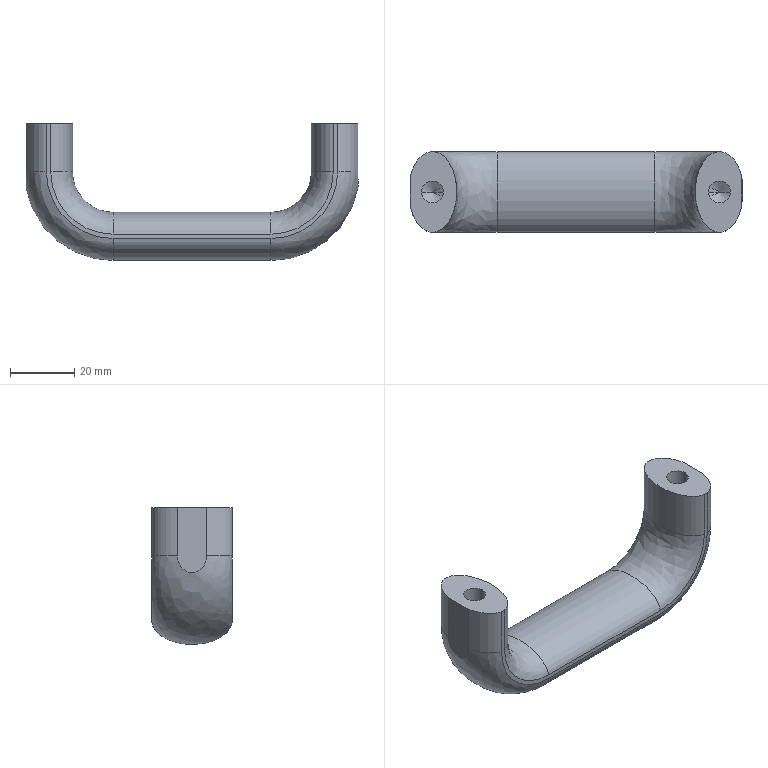Part | SolidWorks | features CutThin 1, HoleWzd 1, Sweep 1 | 1 solid | 26 faces | box 103 x 24.9 x 42.5 mm | volume 40167 mm3 | spline 12 | plane 6 | cylinder 4 | cone 4 | commonest cylinder face diameters 6.8 x4
STEP:
#1=CARTESIAN_POINT('',(-3.4,0.,-19.75));
#2=VERTEX_POINT('',#1);
#3=CARTESIAN_POINT('',(3.4,0.,-19.75));
#4=VERTEX_POINT('',#3);
#5=CARTESIAN_POINT('',(0.,0.,-19.75));
#6=DIRECTION('',(0.,0.,1.));
#7=DIRECTION('',(1.,0.,0.));
#8=AXIS2_PLACEMENT_3D('',#5,#6,#7);
#9=CIRCLE('',#8,3.4);
#10=EDGE_CURVE('',#2,#4,#9,.T.);
#11=ORIENTED_EDGE('',*,*,#10,.F.);
#12=CARTESIAN_POINT('',(-3.4,0.,0.));
#13=VERTEX_POINT('',#12);
#14=CARTESIAN_POINT('',(-3.4,0.,0.));
#15=DIRECTION('',(0.,0.,1.));
#16=VECTOR('',#15,1000.);
#17=LINE('',#14,#16);
#18=EDGE_CURVE('',#2,#13,#17,.T.);
#19=ORIENTED_EDGE('',*,*,#18,.T.);
#20=CARTESIAN_POINT('',(3.4,0.,0.));
#21=VERTEX_POINT('',#20);
#22=CARTESIAN_POINT('',(0.,0.,0.));
#23=DIRECTION('',(0.,0.,1.));
#24=DIRECTION('',(1.,0.,0.));
#25=AXIS2_PLACEMENT_3D('',#22,#23,#24);
#26=CIRCLE('',#25,3.4);
#27=EDGE_CURVE('',#13,#21,#26,.T.);
#28=ORIENTED_EDGE('',*,*,#27,.T.);
#29=CARTESIAN_POINT('',(3.4,0.,0.));
#30=DIRECTION('',(0.,0.,1.));
#31=VECTOR('',#30,1000.);
#32=LINE('',#29,#31);
#33=EDGE_CURVE('',#4,#21,#32,.T.);
#34=ORIENTED_EDGE('',*,*,#33,.F.);
#35=EDGE_LOOP('',(#11,#19,#28,#34));
#36=FACE_OUTER_BOUND('',#35,.T.);
#37=CARTESIAN_POINT('',(0.,0.,0.));
#38=DIRECTION('',(0.,0.,1.));
#39=DIRECTION('',(1.,0.,0.));
#40=AXIS2_PLACEMENT_3D('',#37,#38,#39);
#41=CYLINDRICAL_SURFACE('',#40,3.4);
#42=ADVANCED_FACE('',(#36),#41,.F.);
#43=CARTESIAN_POINT('',(0.,0.,-21.793));
#44=VERTEX_POINT('',#43);
#45=CARTESIAN_POINT('',(3.4,0.,-19.75));
#46=DIRECTION('',(0.8572,0.,0.515));
#47=VECTOR('',#46,1000.);
#48=LINE('',#45,#47);
#49=EDGE_CURVE('',#44,#4,#48,.T.);
#50=ORIENTED_EDGE('',*,*,#49,.F.);
#51=CARTESIAN_POINT('',(-3.4,0.,-19.75));
#52=DIRECTION('',(-0.8572,0.,0.515));
#53=VECTOR('',#52,1000.);
#54=LINE('',#51,#53);
#55=EDGE_CURVE('',#44,#2,#54,.T.);
#56=ORIENTED_EDGE('',*,*,#55,.T.);
#57=ORIENTED_EDGE('',*,*,#10,.T.);
#58=EDGE_LOOP('',(#50,#56,#57));
#59=FACE_OUTER_BOUND('',#58,.T.);
#60=CARTESIAN_POINT('',(0.,0.,-19.75));
#61=DIRECTION('',(0.,0.,1.));
#62=DIRECTION('',(1.,0.,0.));
#63=AXIS2_PLACEMENT_3D('',#60,#61,#62);
#64=CONICAL_SURFACE('',#63,3.4,1.03);
#65=ADVANCED_FACE('',(#59),#64,.F.);
#66=CARTESIAN_POINT('',(85.6,0.,-19.75));
#67=VERTEX_POINT('',#66);
#68=CARTESIAN_POINT('',(92.4,0.,-19.75));
#69=VERTEX_POINT('',#68);
#70=CARTESIAN_POINT('',(89.,0.,-19.75));
#71=DIRECTION('',(0.,0.,1.));
#72=DIRECTION('',(1.,0.,0.));
#73=AXIS2_PLACEMENT_3D('',#70,#71,#72);
#74=CIRCLE('',#73,3.4);
#75=EDGE_CURVE('',#67,#69,#74,.T.);
#76=ORIENTED_EDGE('',*,*,#75,.F.);
#77=CARTESIAN_POINT('',(85.6,0.,0.));
#78=VERTEX_POINT('',#77);
#79=CARTESIAN_POINT('',(85.6,0.,0.));
#80=DIRECTION('',(0.,0.,1.));
#81=VECTOR('',#80,1000.);
#82=LINE('',#79,#81);
#83=EDGE_CURVE('',#67,#78,#82,.T.);
#84=ORIENTED_EDGE('',*,*,#83,.T.);
#85=CARTESIAN_POINT('',(92.4,0.,0.));
#86=VERTEX_POINT('',#85);
#87=CARTESIAN_POINT('',(89.,0.,0.));
#88=DIRECTION('',(0.,0.,1.));
#89=DIRECTION('',(1.,0.,0.));
#90=AXIS2_PLACEMENT_3D('',#87,#88,#89);
#91=CIRCLE('',#90,3.4);
#92=EDGE_CURVE('',#78,#86,#91,.T.);
#93=ORIENTED_EDGE('',*,*,#92,.T.);
#94=CARTESIAN_POINT('',(92.4,0.,0.));
#95=DIRECTION('',(0.,0.,1.));
#96=VECTOR('',#95,1000.);
#97=LINE('',#94,#96);
#98=EDGE_CURVE('',#69,#86,#97,.T.);
#99=ORIENTED_EDGE('',*,*,#98,.F.);
#100=EDGE_LOOP('',(#76,#84,#93,#99));
#101=FACE_OUTER_BOUND('',#100,.T.);
#102=CARTESIAN_POINT('',(89.,0.,0.));
#103=DIRECTION('',(0.,0.,1.));
#104=DIRECTION('',(1.,0.,0.));
#105=AXIS2_PLACEMENT_3D('',#102,#103,#104);
#106=CYLINDRICAL_SURFACE('',#105,3.4);
#107=ADVANCED_FACE('',(#101),#106,.F.);
#108=CARTESIAN_POINT('',(89.,0.,-21.793));
#109=VERTEX_POINT('',#108);
#110=CARTESIAN_POINT('',(92.4,0.,-19.75));
#111=DIRECTION('',(0.8572,0.,0.515));
#112=VECTOR('',#111,1000.);
#113=LINE('',#110,#112);
#114=EDGE_CURVE('',#109,#69,#113,.T.);
#115=ORIENTED_EDGE('',*,*,#114,.F.);
#116=CARTESIAN_POINT('',(85.6,0.,-19.75));
#117=DIRECTION('',(-0.8572,0.,0.515));
#118=VECTOR('',#117,1000.);
#119=LINE('',#116,#118);
#120=EDGE_CURVE('',#109,#67,#119,.T.);
#121=ORIENTED_EDGE('',*,*,#120,.T.);
#122=ORIENTED_EDGE('',*,*,#75,.T.);
#123=EDGE_LOOP('',(#115,#121,#122));
#124=FACE_OUTER_BOUND('',#123,.T.);
#125=CARTESIAN_POINT('',(89.,0.,-19.75));
#126=DIRECTION('',(0.,0.,1.));
#127=DIRECTION('',(1.,0.,0.));
#128=AXIS2_PLACEMENT_3D('',#125,#126,#127);
#129=CONICAL_SURFACE('',#128,3.4,1.03);
#130=ADVANCED_FACE('',(#124),#129,.F.);
#131=CARTESIAN_POINT('',(89.,0.,0.));
#132=DIRECTION('',(0.,0.,1.));
#133=DIRECTION('',(1.,0.,0.));
#134=AXIS2_PLACEMENT_3D('',#131,#132,#133);
#135=CIRCLE('',#134,3.4);
#136=EDGE_CURVE('',#86,#78,#135,.T.);
#137=ORIENTED_EDGE('',*,*,#136,.F.);
#138=ORIENTED_EDGE('',*,*,#92,.F.);
#139=EDGE_LOOP('',(#137,#138));
#140=FACE_BOUND('',#139,.T.);
#141=CARTESIAN_POINT('',(96.,-4.488,0.));
#142=VERTEX_POINT('',#141);
#143=CARTESIAN_POINT('',(96.,4.488,0.));
#144=VERTEX_POINT('',#143);
#145=CARTESIAN_POINT('',(96.,-12.45,0.));
#146=DIRECTION('',(0.,1.,0.));
#147=VECTOR('',#146,1000.);
#148=LINE('',#145,#147);
#149=EDGE_CURVE('',#142,#144,#148,.T.);
#150=ORIENTED_EDGE('',*,*,#149,.T.);
#151=CARTESIAN_POINT('',(89.67,12.45,0.));
#152=VERTEX_POINT('',#151);
#153=CARTESIAN_POINT('',(89.67,12.45,0.));
#154=CARTESIAN_POINT('',(92.598,12.012,0.));
#155=CARTESIAN_POINT('',(94.945,9.061,0.));
#156=CARTESIAN_POINT('',(96.,4.488,0.));
#157=(BOUNDED_CURVE()B_SPLINE_CURVE(3,(#153,#154,#155,#156),.UNSPECIFIED.,.F.,.F.)B_SPLINE_CURVE_WITH_KNOTS((4,4),(0.08947,1.204),.UNSPECIFIED.)CURVE()GEOMETRIC_REPRESENTATION_ITEM()RATIONAL_B_SPLINE_CURVE((1.,0.8992,0.8992,1.))REPRESENTATION_ITEM(''));
#158=EDGE_CURVE('',#152,#144,#157,.T.);
#159=ORIENTED_EDGE('',*,*,#158,.F.);
#160=CARTESIAN_POINT('',(88.33,12.45,0.));
#161=VERTEX_POINT('',#160);
#162=CARTESIAN_POINT('',(-7.,12.45,0.));
#163=DIRECTION('',(-1.,0.,0.));
#164=VECTOR('',#163,1000.);
#165=LINE('',#162,#164);
#166=EDGE_CURVE('',#152,#161,#165,.T.);
#167=ORIENTED_EDGE('',*,*,#166,.T.);
#168=CARTESIAN_POINT('',(88.33,-12.45,0.));
#169=VERTEX_POINT('',#168);
#170=CARTESIAN_POINT('',(88.33,-12.45,0.));
#171=CARTESIAN_POINT('',(75.706,-10.562,0.));
#172=CARTESIAN_POINT('',(75.706,10.562,0.));
#173=CARTESIAN_POINT('',(88.33,12.45,0.));
#174=(BOUNDED_CURVE()B_SPLINE_CURVE(3,(#170,#171,#172,#173),.UNSPECIFIED.,.F.,.F.)B_SPLINE_CURVE_WITH_KNOTS((4,4),(3.231,6.194),.UNSPECIFIED.)CURVE()GEOMETRIC_REPRESENTATION_ITEM()RATIONAL_B_SPLINE_CURVE((1.,0.3929,0.3929,1.))REPRESENTATION_ITEM(''));
#175=EDGE_CURVE('',#169,#161,#174,.T.);
#176=ORIENTED_EDGE('',*,*,#175,.F.);
#177=CARTESIAN_POINT('',(89.67,-12.45,0.));
#178=VERTEX_POINT('',#177);
#179=CARTESIAN_POINT('',(-7.,-12.45,0.));
#180=DIRECTION('',(1.,0.,0.));
#181=VECTOR('',#180,1000.);
#182=LINE('',#179,#181);
#183=EDGE_CURVE('',#169,#178,#182,.T.);
#184=ORIENTED_EDGE('',*,*,#183,.T.);
#185=CARTESIAN_POINT('',(96.,-4.488,0.));
#186=CARTESIAN_POINT('',(94.945,-9.061,0.));
#187=CARTESIAN_POINT('',(92.598,-12.012,0.));
#188=CARTESIAN_POINT('',(89.67,-12.45,0.));
#189=(BOUNDED_CURVE()B_SPLINE_CURVE(3,(#185,#186,#187,#188),.UNSPECIFIED.,.F.,.T.)B_SPLINE_CURVE_WITH_KNOTS((4,4),(1.938,3.052),.UNSPECIFIED.)CURVE()GEOMETRIC_REPRESENTATION_ITEM()RATIONAL_B_SPLINE_CURVE((1.,0.8992,0.8992,1.))REPRESENTATION_ITEM(''));
#190=EDGE_CURVE('',#142,#178,#189,.T.);
#191=ORIENTED_EDGE('',*,*,#190,.F.);
#192=EDGE_LOOP('',(#150,#159,#167,#176,#184,#191));
#193=FACE_OUTER_BOUND('',#192,.T.);
#194=CARTESIAN_POINT('',(89.,0.,0.));
#195=DIRECTION('',(0.,0.,-1.));
#196=DIRECTION('',(-1.,0.,0.));
#197=AXIS2_PLACEMENT_3D('',#194,#195,#196);
#198=PLANE('',#197);
#199=ADVANCED_FACE('',(#140,#193),#198,.F.);
#200=CARTESIAN_POINT('',(0.,0.,0.));
#201=DIRECTION('',(0.,0.,1.));
#202=DIRECTION('',(1.,0.,0.));
#203=AXIS2_PLACEMENT_3D('',#200,#201,#202);
#204=CIRCLE('',#203,3.4);
#205=EDGE_CURVE('',#21,#13,#204,.T.);
#206=ORIENTED_EDGE('',*,*,#205,.F.);
#207=ORIENTED_EDGE('',*,*,#27,.F.);
#208=EDGE_LOOP('',(#206,#207));
#209=FACE_BOUND('',#208,.T.);
#210=CARTESIAN_POINT('',(-7.,-4.488,0.));
#211=VERTEX_POINT('',#210);
#212=CARTESIAN_POINT('',(-0.6701,-12.45,0.));
#213=VERTEX_POINT('',#212);
#214=CARTESIAN_POINT('',(-7.,-4.488,0.));
#215=CARTESIAN_POINT('',(-5.945,-9.061,0.));
#216=CARTESIAN_POINT('',(-3.598,-12.012,0.));
#217=CARTESIAN_POINT('',(-0.6701,-12.45,0.));
#218=(BOUNDED_CURVE()B_SPLINE_CURVE(3,(#214,#215,#216,#217),.UNSPECIFIED.,.F.,.F.)B_SPLINE_CURVE_WITH_KNOTS((4,4),(1.938,3.052),.UNSPECIFIED.)CURVE()GEOMETRIC_REPRESENTATION_ITEM()RATIONAL_B_SPLINE_CURVE((1.,0.8992,0.8992,1.))REPRESENTATION_ITEM(''));
#219=EDGE_CURVE('',#211,#213,#218,.T.);
#220=ORIENTED_EDGE('',*,*,#219,.T.);
#221=CARTESIAN_POINT('',(0.6701,-12.45,0.));
#222=VERTEX_POINT('',#221);
#223=CARTESIAN_POINT('',(-7.,-12.45,0.));
#224=DIRECTION('',(1.,0.,0.));
#225=VECTOR('',#224,1000.);
#226=LINE('',#223,#225);
#227=EDGE_CURVE('',#213,#222,#226,.T.);
#228=ORIENTED_EDGE('',*,*,#227,.T.);
#229=CARTESIAN_POINT('',(0.6701,12.45,0.));
#230=VERTEX_POINT('',#229);
#231=CARTESIAN_POINT('',(0.6701,-12.45,0.));
#232=CARTESIAN_POINT('',(13.294,-10.562,0.));
#233=CARTESIAN_POINT('',(13.294,10.562,0.));
#234=CARTESIAN_POINT('',(0.6701,12.45,0.));
#235=(BOUNDED_CURVE()B_SPLINE_CURVE(3,(#231,#232,#233,#234),.UNSPECIFIED.,.F.,.F.)B_SPLINE_CURVE_WITH_KNOTS((4,4),(3.231,6.194),.UNSPECIFIED.)CURVE()GEOMETRIC_REPRESENTATION_ITEM()RATIONAL_B_SPLINE_CURVE((1.,0.3929,0.3929,1.))REPRESENTATION_ITEM(''));
#236=EDGE_CURVE('',#222,#230,#235,.T.);
#237=ORIENTED_EDGE('',*,*,#236,.T.);
#238=CARTESIAN_POINT('',(-0.6701,12.45,0.));
#239=VERTEX_POINT('',#238);
#240=CARTESIAN_POINT('',(-7.,12.45,0.));
#241=DIRECTION('',(-1.,0.,0.));
#242=VECTOR('',#241,1000.);
#243=LINE('',#240,#242);
#244=EDGE_CURVE('',#230,#239,#243,.T.);
#245=ORIENTED_EDGE('',*,*,#244,.T.);
#246=CARTESIAN_POINT('',(-7.,4.488,0.));
#247=VERTEX_POINT('',#246);
#248=CARTESIAN_POINT('',(-0.6701,12.45,0.));
#249=CARTESIAN_POINT('',(-3.598,12.012,0.));
#250=CARTESIAN_POINT('',(-5.945,9.061,0.));
#251=CARTESIAN_POINT('',(-7.,4.488,0.));
#252=(BOUNDED_CURVE()B_SPLINE_CURVE(3,(#248,#249,#250,#251),.UNSPECIFIED.,.F.,.F.)B_SPLINE_CURVE_WITH_KNOTS((4,4),(0.08947,1.204),.UNSPECIFIED.)CURVE()GEOMETRIC_REPRESENTATION_ITEM()RATIONAL_B_SPLINE_CURVE((1.,0.8992,0.8992,1.))REPRESENTATION_ITEM(''));
#253=EDGE_CURVE('',#239,#247,#252,.T.);
#254=ORIENTED_EDGE('',*,*,#253,.T.);
#255=CARTESIAN_POINT('',(-7.,-12.45,0.));
#256=DIRECTION('',(0.,-1.,0.));
#257=VECTOR('',#256,1000.);
#258=LINE('',#255,#257);
#259=EDGE_CURVE('',#247,#211,#258,.T.);
#260=ORIENTED_EDGE('',*,*,#259,.T.);
#261=EDGE_LOOP('',(#220,#228,#237,#245,#254,#260));
#262=FACE_OUTER_BOUND('',#261,.T.);
#263=CARTESIAN_POINT('',(0.,0.,0.));
#264=DIRECTION('',(0.,0.,1.));
#265=DIRECTION('',(1.,0.,0.));
#266=AXIS2_PLACEMENT_3D('',#263,#264,#265);
#267=PLANE('',#266);
#268=ADVANCED_FACE('',(#209,#262),#267,.T.);
#269=ORIENTED_EDGE('',*,*,#158,.T.);
#270=CARTESIAN_POINT('',(96.,4.488,-15.));
#271=VERTEX_POINT('',#270);
#272=CARTESIAN_POINT('',(96.,4.488,-7.5));
#273=DIRECTION('',(0.,0.,-1.));
#274=VECTOR('',#273,1000.);
#275=LINE('',#272,#274);
#276=EDGE_CURVE('',#144,#271,#275,.T.);
#277=ORIENTED_EDGE('',*,*,#276,.T.);
#278=CARTESIAN_POINT('',(89.67,12.45,-15.));
#279=VERTEX_POINT('',#278);
#280=CARTESIAN_POINT('',(89.67,12.45,-15.));
#281=CARTESIAN_POINT('',(92.598,12.012,-15.));
#282=CARTESIAN_POINT('',(94.945,9.061,-15.));
#283=CARTESIAN_POINT('',(96.,4.488,-15.));
#284=(BOUNDED_CURVE()B_SPLINE_CURVE(3,(#280,#281,#282,#283),.UNSPECIFIED.,.F.,.F.)B_SPLINE_CURVE_WITH_KNOTS((4,4),(0.08947,1.204),.UNSPECIFIED.)CURVE()GEOMETRIC_REPRESENTATION_ITEM()RATIONAL_B_SPLINE_CURVE((1.,0.8992,0.8992,1.))REPRESENTATION_ITEM(''));
#285=EDGE_CURVE('',#279,#271,#284,.T.);
#286=ORIENTED_EDGE('',*,*,#285,.F.);
#287=CARTESIAN_POINT('',(89.67,12.45,-7.5));
#288=DIRECTION('',(0.,0.,1.));
#289=VECTOR('',#288,1000.);
#290=LINE('',#287,#289);
#291=EDGE_CURVE('',#279,#152,#290,.T.);
#292=ORIENTED_EDGE('',*,*,#291,.T.);
#293=EDGE_LOOP('',(#269,#277,#286,#292));
#294=FACE_OUTER_BOUND('',#293,.T.);
#295=CARTESIAN_POINT('',(89.,12.5,0.));
#296=CARTESIAN_POINT('',(89.,12.5,-15.));
#297=CARTESIAN_POINT('',(104.,12.5,0.));
#298=CARTESIAN_POINT('',(104.,12.5,-15.));
#299=CARTESIAN_POINT('',(104.,-12.5,0.));
#300=CARTESIAN_POINT('',(104.,-12.5,-15.));
#301=CARTESIAN_POINT('',(89.,-12.5,0.));
#302=CARTESIAN_POINT('',(89.,-12.5,-15.));
#303=CARTESIAN_POINT('',(74.,-12.5,0.));
#304=CARTESIAN_POINT('',(74.,-12.5,-15.));
#305=CARTESIAN_POINT('',(74.,12.5,0.));
#306=CARTESIAN_POINT('',(74.,12.5,-15.));
#307=CARTESIAN_POINT('',(89.,12.5,0.));
#308=CARTESIAN_POINT('',(89.,12.5,-15.));
#309=(BOUNDED_SURFACE()B_SPLINE_SURFACE(3,1,((#295,#296),(#297,#298),(#299,#300),(#301,#302),(#303,#304),(#305,#306),(#307,#308)),.UNSPECIFIED.,.T.,.F.,.F.)B_SPLINE_SURFACE_WITH_KNOTS((4,3,4),(2,2),(0.,0.5,1.),(0.,1.),.UNSPECIFIED.)GEOMETRIC_REPRESENTATION_ITEM()RATIONAL_B_SPLINE_SURFACE(((1.,1.),(0.3333,0.3333),(0.3333,0.3333),(1.,1.),(0.3333,0.3333),(0.3333,0.3333),(1.,1.)))REPRESENTATION_ITEM('')SURFACE());
#310=ADVANCED_FACE('',(#294),#309,.T.);
#311=CARTESIAN_POINT('',(96.,-4.488,-15.));
#312=VERTEX_POINT('',#311);
#313=CARTESIAN_POINT('',(89.67,-12.45,-15.));
#314=VERTEX_POINT('',#313);
#315=CARTESIAN_POINT('',(96.,-4.488,-15.));
#316=CARTESIAN_POINT('',(94.945,-9.061,-15.));
#317=CARTESIAN_POINT('',(92.598,-12.012,-15.));
#318=CARTESIAN_POINT('',(89.67,-12.45,-15.));
#319=(BOUNDED_CURVE()B_SPLINE_CURVE(3,(#315,#316,#317,#318),.UNSPECIFIED.,.F.,.T.)B_SPLINE_CURVE_WITH_KNOTS((4,4),(1.938,3.052),.UNSPECIFIED.)CURVE()GEOMETRIC_REPRESENTATION_ITEM()RATIONAL_B_SPLINE_CURVE((1.,0.8992,0.8992,1.))REPRESENTATION_ITEM(''));
#320=EDGE_CURVE('',#312,#314,#319,.T.);
#321=ORIENTED_EDGE('',*,*,#320,.F.);
#322=CARTESIAN_POINT('',(96.,-4.488,-7.5));
#323=DIRECTION('',(0.,0.,1.));
#324=VECTOR('',#323,1000.);
#325=LINE('',#322,#324);
#326=EDGE_CURVE('',#312,#142,#325,.T.);
#327=ORIENTED_EDGE('',*,*,#326,.T.);
#328=ORIENTED_EDGE('',*,*,#190,.T.);
#329=CARTESIAN_POINT('',(89.67,-12.45,-7.5));
#330=DIRECTION('',(0.,0.,-1.));
#331=VECTOR('',#330,1000.);
#332=LINE('',#329,#331);
#333=EDGE_CURVE('',#178,#314,#332,.T.);
#334=ORIENTED_EDGE('',*,*,#333,.T.);
#335=EDGE_LOOP('',(#321,#327,#328,#334));
#336=FACE_OUTER_BOUND('',#335,.T.);
#337=CARTESIAN_POINT('',(89.,12.5,0.));
#338=CARTESIAN_POINT('',(89.,12.5,-15.));
#339=CARTESIAN_POINT('',(104.,12.5,0.));
#340=CARTESIAN_POINT('',(104.,12.5,-15.));
#341=CARTESIAN_POINT('',(104.,-12.5,0.));
#342=CARTESIAN_POINT('',(104.,-12.5,-15.));
#343=CARTESIAN_POINT('',(89.,-12.5,0.));
#344=CARTESIAN_POINT('',(89.,-12.5,-15.));
#345=CARTESIAN_POINT('',(74.,-12.5,0.));
#346=CARTESIAN_POINT('',(74.,-12.5,-15.));
#347=CARTESIAN_POINT('',(74.,12.5,0.));
#348=CARTESIAN_POINT('',(74.,12.5,-15.));
#349=CARTESIAN_POINT('',(89.,12.5,0.));
#350=CARTESIAN_POINT('',(89.,12.5,-15.));
#351=(BOUNDED_SURFACE()B_SPLINE_SURFACE(3,1,((#337,#338),(#339,#340),(#341,#342),(#343,#344),(#345,#346),(#347,#348),(#349,#350)),.UNSPECIFIED.,.T.,.F.,.F.)B_SPLINE_SURFACE_WITH_KNOTS((4,3,4),(2,2),(0.,0.5,1.),(0.,1.),.UNSPECIFIED.)GEOMETRIC_REPRESENTATION_ITEM()RATIONAL_B_SPLINE_SURFACE(((1.,1.),(0.3333,0.3333),(0.3333,0.3333),(1.,1.),(0.3333,0.3333),(0.3333,0.3333),(1.,1.)))REPRESENTATION_ITEM('')SURFACE());
#352=ADVANCED_FACE('',(#336),#351,.T.);
#353=CARTESIAN_POINT('',(88.33,-12.45,-15.));
#354=VERTEX_POINT('',#353);
#355=CARTESIAN_POINT('',(88.33,12.45,-15.));
#356=VERTEX_POINT('',#355);
#357=CARTESIAN_POINT('',(88.33,-12.45,-15.));
#358=CARTESIAN_POINT('',(75.706,-10.562,-15.));
#359=CARTESIAN_POINT('',(75.706,10.562,-15.));
#360=CARTESIAN_POINT('',(88.33,12.45,-15.));
#361=(BOUNDED_CURVE()B_SPLINE_CURVE(3,(#357,#358,#359,#360),.UNSPECIFIED.,.F.,.F.)B_SPLINE_CURVE_WITH_KNOTS((4,4),(3.231,6.194),.UNSPECIFIED.)CURVE()GEOMETRIC_REPRESENTATION_ITEM()RATIONAL_B_SPLINE_CURVE((1.,0.3929,0.3929,1.))REPRESENTATION_ITEM(''));
#362=EDGE_CURVE('',#354,#356,#361,.T.);
#363=ORIENTED_EDGE('',*,*,#362,.F.);
#364=CARTESIAN_POINT('',(88.33,-12.45,-7.5));
#365=DIRECTION('',(0.,0.,1.));
#366=VECTOR('',#365,1000.);
#367=LINE('',#364,#366);
#368=EDGE_CURVE('',#354,#169,#367,.T.);
#369=ORIENTED_EDGE('',*,*,#368,.T.);
#370=ORIENTED_EDGE('',*,*,#175,.T.);
#371=CARTESIAN_POINT('',(88.33,12.45,-7.5));
#372=DIRECTION('',(0.,0.,-1.));
#373=VECTOR('',#372,1000.);
#374=LINE('',#371,#373);
#375=EDGE_CURVE('',#161,#356,#374,.T.);
#376=ORIENTED_EDGE('',*,*,#375,.T.);
#377=EDGE_LOOP('',(#363,#369,#370,#376));
#378=FACE_OUTER_BOUND('',#377,.T.);
#379=CARTESIAN_POINT('',(89.,12.5,0.));
#380=CARTESIAN_POINT('',(89.,12.5,-15.));
#381=CARTESIAN_POINT('',(104.,12.5,0.));
#382=CARTESIAN_POINT('',(104.,12.5,-15.));
#383=CARTESIAN_POINT('',(104.,-12.5,0.));
#384=CARTESIAN_POINT('',(104.,-12.5,-15.));
#385=CARTESIAN_POINT('',(89.,-12.5,0.));
#386=CARTESIAN_POINT('',(89.,-12.5,-15.));
#387=CARTESIAN_POINT('',(74.,-12.5,0.));
#388=CARTESIAN_POINT('',(74.,-12.5,-15.));
#389=CARTESIAN_POINT('',(74.,12.5,0.));
#390=CARTESIAN_POINT('',(74.,12.5,-15.));
#391=CARTESIAN_POINT('',(89.,12.5,0.));
#392=CARTESIAN_POINT('',(89.,12.5,-15.));
#393=(BOUNDED_SURFACE()B_SPLINE_SURFACE(3,1,((#379,#380),(#381,#382),(#383,#384),(#385,#386),(#387,#388),(#389,#390),(#391,#392)),.UNSPECIFIED.,.T.,.F.,.T.)B_SPLINE_SURFACE_WITH_KNOTS((4,3,4),(2,2),(0.,0.5,1.),(0.,1.),.UNSPECIFIED.)GEOMETRIC_REPRESENTATION_ITEM()RATIONAL_B_SPLINE_SURFACE(((1.,1.),(0.3333,0.3333),(0.3333,0.3333),(1.,1.),(0.3333,0.3333),(0.3333,0.3333),(1.,1.)))REPRESENTATION_ITEM('')SURFACE());
#394=ADVANCED_FACE('',(#378),#393,.T.);
#395=ORIENTED_EDGE('',*,*,#285,.T.);
#396=CARTESIAN_POINT('',(96.,4.488,-15.));
#397=CARTESIAN_POINT('',(96.,4.488,-15.641));
#398=CARTESIAN_POINT('',(96.,4.392,-16.264));
#399=CARTESIAN_POINT('',(96.,4.1,-17.169));
#400=CARTESIAN_POINT('',(96.,3.976,-17.468));
#401=CARTESIAN_POINT('',(96.,3.681,-18.029));
#402=CARTESIAN_POINT('',(96.,3.511,-18.294));
#403=CARTESIAN_POINT('',(96.,3.12,-18.791));
#404=CARTESIAN_POINT('',(96.,2.895,-19.025));
#405=CARTESIAN_POINT('',(96.,2.407,-19.435));
#406=CARTESIAN_POINT('',(96.,2.144,-19.613));
#407=CARTESIAN_POINT('',(96.,1.717,-19.835));
#408=CARTESIAN_POINT('',(96.,1.57,-19.901));
#409=CARTESIAN_POINT('',(96.,1.272,-20.014));
#410=CARTESIAN_POINT('',(96.,1.121,-20.062));
#411=CARTESIAN_POINT('',(96.,0.8135,-20.139));
#412=CARTESIAN_POINT('',(96.,0.6573,-20.168));
#413=CARTESIAN_POINT('',(96.,0.3397,-20.209));
#414=CARTESIAN_POINT('',(96.,0.1781,-20.219));
#415=CARTESIAN_POINT('',(96.,-0.3005,-20.222));
#416=CARTESIAN_POINT('',(96.,-0.6162,-20.185));
#417=CARTESIAN_POINT('',(96.,-1.241,-20.035));
#418=CARTESIAN_POINT('',(96.,-1.541,-19.923));
#419=CARTESIAN_POINT('',(96.,-2.109,-19.634));
#420=CARTESIAN_POINT('',(96.,-2.38,-19.455));
#421=CARTESIAN_POINT('',(96.,-2.871,-19.048));
#422=CARTESIAN_POINT('',(96.,-3.094,-18.82));
#423=CARTESIAN_POINT('',(96.,-3.495,-18.317));
#424=CARTESIAN_POINT('',(96.,-3.669,-18.05));
#425=CARTESIAN_POINT('',(96.,-3.967,-17.487));
#426=CARTESIAN_POINT('',(96.,-4.093,-17.189));
#427=CARTESIAN_POINT('',(96.,-4.29,-16.583));
#428=CARTESIAN_POINT('',(96.,-4.364,-16.273));
#429=CARTESIAN_POINT('',(96.,-4.463,-15.643));
#430=CARTESIAN_POINT('',(96.,-4.488,-15.321));
#431=CARTESIAN_POINT('',(96.,-4.488,-15.));
#432=B_SPLINE_CURVE_WITH_KNOTS('',3,(#396,#397,#398,#399,#400,#401,#402,#403,#404,#405,#406,#407,#408,#409,#410,#411,#412,#413,#414,#415,#416,#417,#418,#419,#420,#421,#422,#423,#424,#425,#426,#427,#428,#429,#430,#431),.UNSPECIFIED.,.F.,.F.,(4,2,2,2,2,2,2,2,2,2,2,2,2,2,2,2,2,4),(0.,0.001889,0.002833,0.003777,0.004721,0.005666,0.006138,0.00661,0.007082,0.007554,0.008499,0.009443,0.01039,0.01133,0.01228,0.01322,0.01416,0.01511),.UNSPECIFIED.);
#433=EDGE_CURVE('',#271,#312,#432,.T.);
#434=ORIENTED_EDGE('',*,*,#433,.T.);
#435=ORIENTED_EDGE('',*,*,#320,.T.);
#436=CARTESIAN_POINT('',(69.,-12.45,-35.67));
#437=VERTEX_POINT('',#436);
#438=CARTESIAN_POINT('',(69.,-12.45,-15.));
#439=DIRECTION('',(0.,1.,0.));
#440=DIRECTION('',(0.,0.,1.));
#441=AXIS2_PLACEMENT_3D('',#438,#439,#440);
#442=CIRCLE('',#441,20.67);
#443=EDGE_CURVE('',#314,#437,#442,.T.);
#444=ORIENTED_EDGE('',*,*,#443,.T.);
#445=CARTESIAN_POINT('',(69.,12.45,-35.67));
#446=VERTEX_POINT('',#445);
#447=CARTESIAN_POINT('',(69.,12.45,-35.67));
#448=CARTESIAN_POINT('',(69.,10.562,-48.294));
#449=CARTESIAN_POINT('',(69.,-10.562,-48.294));
#450=CARTESIAN_POINT('',(69.,-12.45,-35.67));
#451=(BOUNDED_CURVE()B_SPLINE_CURVE(3,(#447,#448,#449,#450),.UNSPECIFIED.,.F.,.F.)B_SPLINE_CURVE_WITH_KNOTS((4,4),(0.08947,3.052),.UNSPECIFIED.)CURVE()GEOMETRIC_REPRESENTATION_ITEM()RATIONAL_B_SPLINE_CURVE((1.,0.3929,0.3929,1.))REPRESENTATION_ITEM(''));
#452=EDGE_CURVE('',#446,#437,#451,.T.);
#453=ORIENTED_EDGE('',*,*,#452,.F.);
#454=CARTESIAN_POINT('',(69.,12.45,-15.));
#455=DIRECTION('',(0.,-1.,0.));
#456=DIRECTION('',(0.,0.,1.));
#457=AXIS2_PLACEMENT_3D('',#454,#455,#456);
#458=CIRCLE('',#457,20.67);
#459=EDGE_CURVE('',#446,#279,#458,.T.);
#460=ORIENTED_EDGE('',*,*,#459,.T.);
#461=EDGE_LOOP('',(#395,#434,#435,#444,#453,#460));
#462=FACE_OUTER_BOUND('',#461,.T.);
#463=CARTESIAN_POINT('',(89.,12.5,-15.));
#464=CARTESIAN_POINT('',(89.,12.5,-26.716));
#465=CARTESIAN_POINT('',(80.716,12.5,-35.));
#466=CARTESIAN_POINT('',(69.,12.5,-35.));
#467=CARTESIAN_POINT('',(104.,12.5,-15.));
#468=CARTESIAN_POINT('',(104.,12.5,-35.503));
#469=CARTESIAN_POINT('',(89.503,12.5,-50.));
#470=CARTESIAN_POINT('',(69.,12.5,-50.));
#471=CARTESIAN_POINT('',(104.,-12.5,-15.));
#472=CARTESIAN_POINT('',(104.,-12.5,-35.503));
#473=CARTESIAN_POINT('',(89.503,-12.5,-50.));
#474=CARTESIAN_POINT('',(69.,-12.5,-50.));
#475=CARTESIAN_POINT('',(89.,-12.5,-15.));
#476=CARTESIAN_POINT('',(89.,-12.5,-26.716));
#477=CARTESIAN_POINT('',(80.716,-12.5,-35.));
#478=CARTESIAN_POINT('',(69.,-12.5,-35.));
#479=CARTESIAN_POINT('',(74.,-12.5,-15.));
#480=CARTESIAN_POINT('',(74.,-12.5,-17.929));
#481=CARTESIAN_POINT('',(71.929,-12.5,-20.));
#482=CARTESIAN_POINT('',(69.,-12.5,-20.));
#483=CARTESIAN_POINT('',(74.,12.5,-15.));
#484=CARTESIAN_POINT('',(74.,12.5,-17.929));
#485=CARTESIAN_POINT('',(71.929,12.5,-20.));
#486=CARTESIAN_POINT('',(69.,12.5,-20.));
#487=CARTESIAN_POINT('',(89.,12.5,-15.));
#488=CARTESIAN_POINT('',(89.,12.5,-26.716));
#489=CARTESIAN_POINT('',(80.716,12.5,-35.));
#490=CARTESIAN_POINT('',(69.,12.5,-35.));
#491=(BOUNDED_SURFACE()B_SPLINE_SURFACE(3,3,((#463,#464,#465,#466),(#467,#468,#469,#470),(#471,#472,#473,#474),(#475,#476,#477,#478),(#479,#480,#481,#482),(#483,#484,#485,#486),(#487,#488,#489,#490)),.UNSPECIFIED.,.T.,.F.,.F.)B_SPLINE_SURFACE_WITH_KNOTS((4,3,4),(4,4),(0.,0.5,1.),(0.,1.),.UNSPECIFIED.)GEOMETRIC_REPRESENTATION_ITEM()RATIONAL_B_SPLINE_SURFACE(((1.,0.8047,0.8047,1.),(0.3333,0.2682,0.2682,0.3333),(0.3333,0.2682,0.2682,0.3333),(1.,0.8047,0.8047,1.),(0.3333,0.2682,0.2682,0.3333),(0.3333,0.2682,0.2682,0.3333),(1.,0.8047,0.8047,1.)))REPRESENTATION_ITEM('')SURFACE());
#492=ADVANCED_FACE('',(#462),#491,.T.);
#493=CARTESIAN_POINT('',(69.,-12.45,-34.33));
#494=VERTEX_POINT('',#493);
#495=CARTESIAN_POINT('',(69.,12.45,-34.33));
#496=VERTEX_POINT('',#495);
#497=CARTESIAN_POINT('',(69.,-12.45,-34.33));
#498=CARTESIAN_POINT('',(69.,-10.562,-21.706));
#499=CARTESIAN_POINT('',(69.,10.562,-21.706));
#500=CARTESIAN_POINT('',(69.,12.45,-34.33));
#501=(BOUNDED_CURVE()B_SPLINE_CURVE(3,(#497,#498,#499,#500),.UNSPECIFIED.,.F.,.F.)B_SPLINE_CURVE_WITH_KNOTS((4,4),(3.231,6.194),.UNSPECIFIED.)CURVE()GEOMETRIC_REPRESENTATION_ITEM()RATIONAL_B_SPLINE_CURVE((1.,0.3929,0.3929,1.))REPRESENTATION_ITEM(''));
#502=EDGE_CURVE('',#494,#496,#501,.T.);
#503=ORIENTED_EDGE('',*,*,#502,.F.);
#504=CARTESIAN_POINT('',(69.,-12.45,-15.));
#505=DIRECTION('',(0.,-1.,0.));
#506=DIRECTION('',(0.,0.,1.));
#507=AXIS2_PLACEMENT_3D('',#504,#505,#506);
#508=CIRCLE('',#507,19.33);
#509=EDGE_CURVE('',#494,#354,#508,.T.);
#510=ORIENTED_EDGE('',*,*,#509,.T.);
#511=ORIENTED_EDGE('',*,*,#362,.T.);
#512=CARTESIAN_POINT('',(69.,12.45,-15.));
#513=DIRECTION('',(0.,1.,0.));
#514=DIRECTION('',(0.,0.,1.));
#515=AXIS2_PLACEMENT_3D('',#512,#513,#514);
#516=CIRCLE('',#515,19.33);
#517=EDGE_CURVE('',#356,#496,#516,.T.);
#518=ORIENTED_EDGE('',*,*,#517,.T.);
#519=EDGE_LOOP('',(#503,#510,#511,#518));
#520=FACE_OUTER_BOUND('',#519,.T.);
#521=CARTESIAN_POINT('',(89.,12.5,-15.));
#522=CARTESIAN_POINT('',(89.,12.5,-26.716));
#523=CARTESIAN_POINT('',(80.716,12.5,-35.));
#524=CARTESIAN_POINT('',(69.,12.5,-35.));
#525=CARTESIAN_POINT('',(104.,12.5,-15.));
#526=CARTESIAN_POINT('',(104.,12.5,-35.503));
#527=CARTESIAN_POINT('',(89.503,12.5,-50.));
#528=CARTESIAN_POINT('',(69.,12.5,-50.));
#529=CARTESIAN_POINT('',(104.,-12.5,-15.));
#530=CARTESIAN_POINT('',(104.,-12.5,-35.503));
#531=CARTESIAN_POINT('',(89.503,-12.5,-50.));
#532=CARTESIAN_POINT('',(69.,-12.5,-50.));
#533=CARTESIAN_POINT('',(89.,-12.5,-15.));
#534=CARTESIAN_POINT('',(89.,-12.5,-26.716));
#535=CARTESIAN_POINT('',(80.716,-12.5,-35.));
#536=CARTESIAN_POINT('',(69.,-12.5,-35.));
#537=CARTESIAN_POINT('',(74.,-12.5,-15.));
#538=CARTESIAN_POINT('',(74.,-12.5,-17.929));
#539=CARTESIAN_POINT('',(71.929,-12.5,-20.));
#540=CARTESIAN_POINT('',(69.,-12.5,-20.));
#541=CARTESIAN_POINT('',(74.,12.5,-15.));
#542=CARTESIAN_POINT('',(74.,12.5,-17.929));
#543=CARTESIAN_POINT('',(71.929,12.5,-20.));
#544=CARTESIAN_POINT('',(69.,12.5,-20.));
#545=CARTESIAN_POINT('',(89.,12.5,-15.));
#546=CARTESIAN_POINT('',(89.,12.5,-26.716));
#547=CARTESIAN_POINT('',(80.716,12.5,-35.));
#548=CARTESIAN_POINT('',(69.,12.5,-35.));
#549=(BOUNDED_SURFACE()B_SPLINE_SURFACE(3,3,((#521,#522,#523,#524),(#525,#526,#527,#528),(#529,#530,#531,#532),(#533,#534,#535,#536),(#537,#538,#539,#540),(#541,#542,#543,#544),(#545,#546,#547,#548)),.UNSPECIFIED.,.T.,.F.,.T.)B_SPLINE_SURFACE_WITH_KNOTS((4,3,4),(4,4),(0.,0.5,1.),(0.,1.),.UNSPECIFIED.)GEOMETRIC_REPRESENTATION_ITEM()RATIONAL_B_SPLINE_SURFACE(((1.,0.8047,0.8047,1.),(0.3333,0.2682,0.2682,0.3333),(0.3333,0.2682,0.2682,0.3333),(1.,0.8047,0.8047,1.),(0.3333,0.2682,0.2682,0.3333),(0.3333,0.2682,0.2682,0.3333),(1.,0.8047,0.8047,1.)))REPRESENTATION_ITEM('')SURFACE());
#550=ADVANCED_FACE('',(#520),#549,.T.);
#551=ORIENTED_EDGE('',*,*,#452,.T.);
#552=CARTESIAN_POINT('',(20.,-12.45,-35.67));
#553=VERTEX_POINT('',#552);
#554=CARTESIAN_POINT('',(44.5,-12.45,-35.67));
#555=DIRECTION('',(-1.,0.,0.));
#556=VECTOR('',#555,1000.);
#557=LINE('',#554,#556);
#558=EDGE_CURVE('',#437,#553,#557,.T.);
#559=ORIENTED_EDGE('',*,*,#558,.T.);
#560=CARTESIAN_POINT('',(20.,12.45,-35.67));
#561=VERTEX_POINT('',#560);
#562=CARTESIAN_POINT('',(20.,12.45,-35.67));
#563=CARTESIAN_POINT('',(20.,10.562,-48.294));
#564=CARTESIAN_POINT('',(20.,-10.562,-48.294));
#565=CARTESIAN_POINT('',(20.,-12.45,-35.67));
#566=(BOUNDED_CURVE()B_SPLINE_CURVE(3,(#562,#563,#564,#565),.UNSPECIFIED.,.F.,.F.)B_SPLINE_CURVE_WITH_KNOTS((4,4),(0.08947,3.052),.UNSPECIFIED.)CURVE()GEOMETRIC_REPRESENTATION_ITEM()RATIONAL_B_SPLINE_CURVE((1.,0.3929,0.3929,1.))REPRESENTATION_ITEM(''));
#567=EDGE_CURVE('',#561,#553,#566,.T.);
#568=ORIENTED_EDGE('',*,*,#567,.F.);
#569=CARTESIAN_POINT('',(44.5,12.45,-35.67));
#570=DIRECTION('',(1.,0.,0.));
#571=VECTOR('',#570,1000.);
#572=LINE('',#569,#571);
#573=EDGE_CURVE('',#561,#446,#572,.T.);
#574=ORIENTED_EDGE('',*,*,#573,.T.);
#575=EDGE_LOOP('',(#551,#559,#568,#574));
#576=FACE_OUTER_BOUND('',#575,.T.);
#577=CARTESIAN_POINT('',(69.,12.5,-35.));
#578=CARTESIAN_POINT('',(20.,12.5,-35.));
#579=CARTESIAN_POINT('',(69.,12.5,-50.));
#580=CARTESIAN_POINT('',(20.,12.5,-50.));
#581=CARTESIAN_POINT('',(69.,-12.5,-50.));
#582=CARTESIAN_POINT('',(20.,-12.5,-50.));
#583=CARTESIAN_POINT('',(69.,-12.5,-35.));
#584=CARTESIAN_POINT('',(20.,-12.5,-35.));
#585=CARTESIAN_POINT('',(69.,-12.5,-20.));
#586=CARTESIAN_POINT('',(20.,-12.5,-20.));
#587=CARTESIAN_POINT('',(69.,12.5,-20.));
#588=CARTESIAN_POINT('',(20.,12.5,-20.));
#589=CARTESIAN_POINT('',(69.,12.5,-35.));
#590=CARTESIAN_POINT('',(20.,12.5,-35.));
#591=(BOUNDED_SURFACE()B_SPLINE_SURFACE(3,1,((#577,#578),(#579,#580),(#581,#582),(#583,#584),(#585,#586),(#587,#588),(#589,#590)),.UNSPECIFIED.,.T.,.F.,.F.)B_SPLINE_SURFACE_WITH_KNOTS((4,3,4),(2,2),(0.,0.5,1.),(0.,1.),.UNSPECIFIED.)GEOMETRIC_REPRESENTATION_ITEM()RATIONAL_B_SPLINE_SURFACE(((1.,1.),(0.3333,0.3333),(0.3333,0.3333),(1.,1.),(0.3333,0.3333),(0.3333,0.3333),(1.,1.)))REPRESENTATION_ITEM('')SURFACE());
#592=ADVANCED_FACE('',(#576),#591,.T.);
#593=CARTESIAN_POINT('',(20.,-12.45,-34.33));
#594=VERTEX_POINT('',#593);
#595=CARTESIAN_POINT('',(20.,12.45,-34.33));
#596=VERTEX_POINT('',#595);
#597=CARTESIAN_POINT('',(20.,-12.45,-34.33));
#598=CARTESIAN_POINT('',(20.,-10.562,-21.706));
#599=CARTESIAN_POINT('',(20.,10.562,-21.706));
#600=CARTESIAN_POINT('',(20.,12.45,-34.33));
#601=(BOUNDED_CURVE()B_SPLINE_CURVE(3,(#597,#598,#599,#600),.UNSPECIFIED.,.F.,.F.)B_SPLINE_CURVE_WITH_KNOTS((4,4),(3.231,6.194),.UNSPECIFIED.)CURVE()GEOMETRIC_REPRESENTATION_ITEM()RATIONAL_B_SPLINE_CURVE((1.,0.3929,0.3929,1.))REPRESENTATION_ITEM(''));
#602=EDGE_CURVE('',#594,#596,#601,.T.);
#603=ORIENTED_EDGE('',*,*,#602,.F.);
#604=CARTESIAN_POINT('',(44.5,-12.45,-34.33));
#605=DIRECTION('',(1.,0.,0.));
#606=VECTOR('',#605,1000.);
#607=LINE('',#604,#606);
#608=EDGE_CURVE('',#594,#494,#607,.T.);
#609=ORIENTED_EDGE('',*,*,#608,.T.);
#610=ORIENTED_EDGE('',*,*,#502,.T.);
#611=CARTESIAN_POINT('',(44.5,12.45,-34.33));
#612=DIRECTION('',(-1.,0.,0.));
#613=VECTOR('',#612,1000.);
#614=LINE('',#611,#613);
#615=EDGE_CURVE('',#496,#596,#614,.T.);
#616=ORIENTED_EDGE('',*,*,#615,.T.);
#617=EDGE_LOOP('',(#603,#609,#610,#616));
#618=FACE_OUTER_BOUND('',#617,.T.);
#619=CARTESIAN_POINT('',(69.,12.5,-35.));
#620=CARTESIAN_POINT('',(20.,12.5,-35.));
#621=CARTESIAN_POINT('',(69.,12.5,-50.));
#622=CARTESIAN_POINT('',(20.,12.5,-50.));
#623=CARTESIAN_POINT('',(69.,-12.5,-50.));
#624=CARTESIAN_POINT('',(20.,-12.5,-50.));
#625=CARTESIAN_POINT('',(69.,-12.5,-35.));
#626=CARTESIAN_POINT('',(20.,-12.5,-35.));
#627=CARTESIAN_POINT('',(69.,-12.5,-20.));
#628=CARTESIAN_POINT('',(20.,-12.5,-20.));
#629=CARTESIAN_POINT('',(69.,12.5,-20.));
#630=CARTESIAN_POINT('',(20.,12.5,-20.));
#631=CARTESIAN_POINT('',(69.,12.5,-35.));
#632=CARTESIAN_POINT('',(20.,12.5,-35.));
#633=(BOUNDED_SURFACE()B_SPLINE_SURFACE(3,1,((#619,#620),(#621,#622),(#623,#624),(#625,#626),(#627,#628),(#629,#630),(#631,#632)),.UNSPECIFIED.,.T.,.F.,.F.)B_SPLINE_SURFACE_WITH_KNOTS((4,3,4),(2,2),(0.,0.5,1.),(0.,1.),.UNSPECIFIED.)GEOMETRIC_REPRESENTATION_ITEM()RATIONAL_B_SPLINE_SURFACE(((1.,1.),(0.3333,0.3333),(0.3333,0.3333),(1.,1.),(0.3333,0.3333),(0.3333,0.3333),(1.,1.)))REPRESENTATION_ITEM('')SURFACE());
#634=ADVANCED_FACE('',(#618),#633,.T.);
#635=ORIENTED_EDGE('',*,*,#567,.T.);
#636=CARTESIAN_POINT('',(-0.6701,-12.45,-15.));
#637=VERTEX_POINT('',#636);
#638=CARTESIAN_POINT('',(20.,-12.45,-15.));
#639=DIRECTION('',(0.,1.,0.));
#640=DIRECTION('',(0.,0.,1.));
#641=AXIS2_PLACEMENT_3D('',#638,#639,#640);
#642=CIRCLE('',#641,20.67);
#643=EDGE_CURVE('',#553,#637,#642,.T.);
#644=ORIENTED_EDGE('',*,*,#643,.T.);
#645=CARTESIAN_POINT('',(-7.,-4.488,-15.));
#646=VERTEX_POINT('',#645);
#647=CARTESIAN_POINT('',(-7.,-4.488,-15.));
#648=CARTESIAN_POINT('',(-5.945,-9.061,-15.));
#649=CARTESIAN_POINT('',(-3.598,-12.012,-15.));
#650=CARTESIAN_POINT('',(-0.6701,-12.45,-15.));
#651=(BOUNDED_CURVE()B_SPLINE_CURVE(3,(#647,#648,#649,#650),.UNSPECIFIED.,.F.,.T.)B_SPLINE_CURVE_WITH_KNOTS((4,4),(1.938,3.052),.UNSPECIFIED.)CURVE()GEOMETRIC_REPRESENTATION_ITEM()RATIONAL_B_SPLINE_CURVE((1.,0.8992,0.8992,1.))REPRESENTATION_ITEM(''));
#652=EDGE_CURVE('',#646,#637,#651,.T.);
#653=ORIENTED_EDGE('',*,*,#652,.F.);
#654=CARTESIAN_POINT('',(-7.,4.488,-15.));
#655=VERTEX_POINT('',#654);
#656=CARTESIAN_POINT('',(-7.,-4.488,-15.));
#657=CARTESIAN_POINT('',(-7.,-4.488,-15.641));
#658=CARTESIAN_POINT('',(-7.,-4.392,-16.264));
#659=CARTESIAN_POINT('',(-7.,-4.1,-17.169));
#660=CARTESIAN_POINT('',(-7.,-3.976,-17.468));
#661=CARTESIAN_POINT('',(-7.,-3.681,-18.029));
#662=CARTESIAN_POINT('',(-7.,-3.511,-18.294));
#663=CARTESIAN_POINT('',(-7.,-3.12,-18.791));
#664=CARTESIAN_POINT('',(-7.,-2.895,-19.025));
#665=CARTESIAN_POINT('',(-7.,-2.407,-19.435));
#666=CARTESIAN_POINT('',(-7.,-2.144,-19.613));
#667=CARTESIAN_POINT('',(-7.,-1.717,-19.835));
#668=CARTESIAN_POINT('',(-7.,-1.57,-19.901));
#669=CARTESIAN_POINT('',(-7.,-1.272,-20.014));
#670=CARTESIAN_POINT('',(-7.,-1.121,-20.062));
#671=CARTESIAN_POINT('',(-7.,-0.8135,-20.139));
#672=CARTESIAN_POINT('',(-7.,-0.6573,-20.168));
#673=CARTESIAN_POINT('',(-7.,-0.3397,-20.209));
#674=CARTESIAN_POINT('',(-7.,-0.1781,-20.219));
#675=CARTESIAN_POINT('',(-7.,0.3005,-20.222));
#676=CARTESIAN_POINT('',(-7.,0.6162,-20.185));
#677=CARTESIAN_POINT('',(-7.,1.241,-20.035));
#678=CARTESIAN_POINT('',(-7.,1.541,-19.923));
#679=CARTESIAN_POINT('',(-7.,2.109,-19.634));
#680=CARTESIAN_POINT('',(-7.,2.38,-19.455));
#681=CARTESIAN_POINT('',(-7.,2.871,-19.048));
#682=CARTESIAN_POINT('',(-7.,3.094,-18.82));
#683=CARTESIAN_POINT('',(-7.,3.495,-18.317));
#684=CARTESIAN_POINT('',(-7.,3.669,-18.05));
#685=CARTESIAN_POINT('',(-7.,3.967,-17.487));
#686=CARTESIAN_POINT('',(-7.,4.093,-17.189));
#687=CARTESIAN_POINT('',(-7.,4.29,-16.583));
#688=CARTESIAN_POINT('',(-7.,4.364,-16.273));
#689=CARTESIAN_POINT('',(-7.,4.463,-15.643));
#690=CARTESIAN_POINT('',(-7.,4.488,-15.321));
#691=CARTESIAN_POINT('',(-7.,4.488,-15.));
#692=B_SPLINE_CURVE_WITH_KNOTS('',3,(#656,#657,#658,#659,#660,#661,#662,#663,#664,#665,#666,#667,#668,#669,#670,#671,#672,#673,#674,#675,#676,#677,#678,#679,#680,#681,#682,#683,#684,#685,#686,#687,#688,#689,#690,#691),.UNSPECIFIED.,.F.,.F.,(4,2,2,2,2,2,2,2,2,2,2,2,2,2,2,2,2,4),(0.,0.001889,0.002833,0.003777,0.004721,0.005666,0.006138,0.00661,0.007082,0.007554,0.008499,0.009443,0.01039,0.01133,0.01228,0.01322,0.01416,0.01511),.UNSPECIFIED.);
#693=EDGE_CURVE('',#646,#655,#692,.T.);
#694=ORIENTED_EDGE('',*,*,#693,.T.);
#695=CARTESIAN_POINT('',(-0.6701,12.45,-15.));
#696=VERTEX_POINT('',#695);
#697=CARTESIAN_POINT('',(-0.6701,12.45,-15.));
#698=CARTESIAN_POINT('',(-3.598,12.012,-15.));
#699=CARTESIAN_POINT('',(-5.945,9.061,-15.));
#700=CARTESIAN_POINT('',(-7.,4.488,-15.));
#701=(BOUNDED_CURVE()B_SPLINE_CURVE(3,(#697,#698,#699,#700),.UNSPECIFIED.,.F.,.F.)B_SPLINE_CURVE_WITH_KNOTS((4,4),(0.08947,1.204),.UNSPECIFIED.)CURVE()GEOMETRIC_REPRESENTATION_ITEM()RATIONAL_B_SPLINE_CURVE((1.,0.8992,0.8992,1.))REPRESENTATION_ITEM(''));
#702=EDGE_CURVE('',#696,#655,#701,.T.);
#703=ORIENTED_EDGE('',*,*,#702,.F.);
#704=CARTESIAN_POINT('',(20.,12.45,-15.));
#705=DIRECTION('',(0.,-1.,0.));
#706=DIRECTION('',(0.,0.,1.));
#707=AXIS2_PLACEMENT_3D('',#704,#705,#706);
#708=CIRCLE('',#707,20.67);
#709=EDGE_CURVE('',#696,#561,#708,.T.);
#710=ORIENTED_EDGE('',*,*,#709,.T.);
#711=EDGE_LOOP('',(#635,#644,#653,#694,#703,#710));
#712=FACE_OUTER_BOUND('',#711,.T.);
#713=CARTESIAN_POINT('',(20.,12.5,-35.));
#714=CARTESIAN_POINT('',(8.284,12.5,-35.));
#715=CARTESIAN_POINT('',(0.,12.5,-26.716));
#716=CARTESIAN_POINT('',(0.,12.5,-15.));
#717=CARTESIAN_POINT('',(20.,12.5,-50.));
#718=CARTESIAN_POINT('',(-0.5025,12.5,-50.));
#719=CARTESIAN_POINT('',(-15.,12.5,-35.503));
#720=CARTESIAN_POINT('',(-15.,12.5,-15.));
#721=CARTESIAN_POINT('',(20.,-12.5,-50.));
#722=CARTESIAN_POINT('',(-0.5025,-12.5,-50.));
#723=CARTESIAN_POINT('',(-15.,-12.5,-35.503));
#724=CARTESIAN_POINT('',(-15.,-12.5,-15.));
#725=CARTESIAN_POINT('',(20.,-12.5,-35.));
#726=CARTESIAN_POINT('',(8.284,-12.5,-35.));
#727=CARTESIAN_POINT('',(0.,-12.5,-26.716));
#728=CARTESIAN_POINT('',(0.,-12.5,-15.));
#729=CARTESIAN_POINT('',(20.,-12.5,-20.));
#730=CARTESIAN_POINT('',(17.071,-12.5,-20.));
#731=CARTESIAN_POINT('',(15.,-12.5,-17.929));
#732=CARTESIAN_POINT('',(15.,-12.5,-15.));
#733=CARTESIAN_POINT('',(20.,12.5,-20.));
#734=CARTESIAN_POINT('',(17.071,12.5,-20.));
#735=CARTESIAN_POINT('',(15.,12.5,-17.929));
#736=CARTESIAN_POINT('',(15.,12.5,-15.));
#737=CARTESIAN_POINT('',(20.,12.5,-35.));
#738=CARTESIAN_POINT('',(8.284,12.5,-35.));
#739=CARTESIAN_POINT('',(0.,12.5,-26.716));
#740=CARTESIAN_POINT('',(0.,12.5,-15.));
#741=(BOUNDED_SURFACE()B_SPLINE_SURFACE(3,3,((#713,#714,#715,#716),(#717,#718,#719,#720),(#721,#722,#723,#724),(#725,#726,#727,#728),(#729,#730,#731,#732),(#733,#734,#735,#736),(#737,#738,#739,#740)),.UNSPECIFIED.,.T.,.F.,.T.)B_SPLINE_SURFACE_WITH_KNOTS((4,3,4),(4,4),(0.,0.5,1.),(0.,1.),.UNSPECIFIED.)GEOMETRIC_REPRESENTATION_ITEM()RATIONAL_B_SPLINE_SURFACE(((1.,0.8047,0.8047,1.),(0.3333,0.2682,0.2682,0.3333),(0.3333,0.2682,0.2682,0.3333),(1.,0.8047,0.8047,1.),(0.3333,0.2682,0.2682,0.3333),(0.3333,0.2682,0.2682,0.3333),(1.,0.8047,0.8047,1.)))REPRESENTATION_ITEM('')SURFACE());
#742=ADVANCED_FACE('',(#712),#741,.T.);
#743=CARTESIAN_POINT('',(0.6701,-12.45,-15.));
#744=VERTEX_POINT('',#743);
#745=CARTESIAN_POINT('',(0.6701,12.45,-15.));
#746=VERTEX_POINT('',#745);
#747=CARTESIAN_POINT('',(0.6701,-12.45,-15.));
#748=CARTESIAN_POINT('',(13.294,-10.562,-15.));
#749=CARTESIAN_POINT('',(13.294,10.562,-15.));
#750=CARTESIAN_POINT('',(0.6701,12.45,-15.));
#751=(BOUNDED_CURVE()B_SPLINE_CURVE(3,(#747,#748,#749,#750),.UNSPECIFIED.,.F.,.T.)B_SPLINE_CURVE_WITH_KNOTS((4,4),(3.231,6.194),.UNSPECIFIED.)CURVE()GEOMETRIC_REPRESENTATION_ITEM()RATIONAL_B_SPLINE_CURVE((1.,0.3929,0.3929,1.))REPRESENTATION_ITEM(''));
#752=EDGE_CURVE('',#744,#746,#751,.T.);
#753=ORIENTED_EDGE('',*,*,#752,.F.);
#754=CARTESIAN_POINT('',(20.,-12.45,-15.));
#755=DIRECTION('',(0.,-1.,0.));
#756=DIRECTION('',(0.,0.,1.));
#757=AXIS2_PLACEMENT_3D('',#754,#755,#756);
#758=CIRCLE('',#757,19.33);
#759=EDGE_CURVE('',#744,#594,#758,.T.);
#760=ORIENTED_EDGE('',*,*,#759,.T.);
#761=ORIENTED_EDGE('',*,*,#602,.T.);
#762=CARTESIAN_POINT('',(20.,12.45,-15.));
#763=DIRECTION('',(0.,1.,0.));
#764=DIRECTION('',(0.,0.,1.));
#765=AXIS2_PLACEMENT_3D('',#762,#763,#764);
#766=CIRCLE('',#765,19.33);
#767=EDGE_CURVE('',#596,#746,#766,.T.);
#768=ORIENTED_EDGE('',*,*,#767,.T.);
#769=EDGE_LOOP('',(#753,#760,#761,#768));
#770=FACE_OUTER_BOUND('',#769,.T.);
#771=CARTESIAN_POINT('',(20.,12.5,-35.));
#772=CARTESIAN_POINT('',(8.284,12.5,-35.));
#773=CARTESIAN_POINT('',(0.,12.5,-26.716));
#774=CARTESIAN_POINT('',(0.,12.5,-15.));
#775=CARTESIAN_POINT('',(20.,12.5,-50.));
#776=CARTESIAN_POINT('',(-0.5025,12.5,-50.));
#777=CARTESIAN_POINT('',(-15.,12.5,-35.503));
#778=CARTESIAN_POINT('',(-15.,12.5,-15.));
#779=CARTESIAN_POINT('',(20.,-12.5,-50.));
#780=CARTESIAN_POINT('',(-0.5025,-12.5,-50.));
#781=CARTESIAN_POINT('',(-15.,-12.5,-35.503));
#782=CARTESIAN_POINT('',(-15.,-12.5,-15.));
#783=CARTESIAN_POINT('',(20.,-12.5,-35.));
#784=CARTESIAN_POINT('',(8.284,-12.5,-35.));
#785=CARTESIAN_POINT('',(0.,-12.5,-26.716));
#786=CARTESIAN_POINT('',(0.,-12.5,-15.));
#787=CARTESIAN_POINT('',(20.,-12.5,-20.));
#788=CARTESIAN_POINT('',(17.071,-12.5,-20.));
#789=CARTESIAN_POINT('',(15.,-12.5,-17.929));
#790=CARTESIAN_POINT('',(15.,-12.5,-15.));
#791=CARTESIAN_POINT('',(20.,12.5,-20.));
#792=CARTESIAN_POINT('',(17.071,12.5,-20.));
#793=CARTESIAN_POINT('',(15.,12.5,-17.929));
#794=CARTESIAN_POINT('',(15.,12.5,-15.));
#795=CARTESIAN_POINT('',(20.,12.5,-35.));
#796=CARTESIAN_POINT('',(8.284,12.5,-35.));
#797=CARTESIAN_POINT('',(0.,12.5,-26.716));
#798=CARTESIAN_POINT('',(0.,12.5,-15.));
#799=(BOUNDED_SURFACE()B_SPLINE_SURFACE(3,3,((#771,#772,#773,#774),(#775,#776,#777,#778),(#779,#780,#781,#782),(#783,#784,#785,#786),(#787,#788,#789,#790),(#791,#792,#793,#794),(#795,#796,#797,#798)),.UNSPECIFIED.,.T.,.F.,.F.)B_SPLINE_SURFACE_WITH_KNOTS((4,3,4),(4,4),(0.,0.5,1.),(0.,1.),.UNSPECIFIED.)GEOMETRIC_REPRESENTATION_ITEM()RATIONAL_B_SPLINE_SURFACE(((1.,0.8047,0.8047,1.),(0.3333,0.2682,0.2682,0.3333),(0.3333,0.2682,0.2682,0.3333),(1.,0.8047,0.8047,1.),(0.3333,0.2682,0.2682,0.3333),(0.3333,0.2682,0.2682,0.3333),(1.,0.8047,0.8047,1.)))REPRESENTATION_ITEM('')SURFACE());
#800=ADVANCED_FACE('',(#770),#799,.T.);
#801=ORIENTED_EDGE('',*,*,#652,.T.);
#802=CARTESIAN_POINT('',(-0.6701,-12.45,-7.5));
#803=DIRECTION('',(0.,0.,1.));
#804=VECTOR('',#803,1000.);
#805=LINE('',#802,#804);
#806=EDGE_CURVE('',#637,#213,#805,.T.);
#807=ORIENTED_EDGE('',*,*,#806,.T.);
#808=ORIENTED_EDGE('',*,*,#219,.F.);
#809=CARTESIAN_POINT('',(-7.,-4.488,-7.5));
#810=DIRECTION('',(0.,0.,-1.));
#811=VECTOR('',#810,1000.);
#812=LINE('',#809,#811);
#813=EDGE_CURVE('',#211,#646,#812,.T.);
#814=ORIENTED_EDGE('',*,*,#813,.T.);
#815=EDGE_LOOP('',(#801,#807,#808,#814));
#816=FACE_OUTER_BOUND('',#815,.T.);
#817=CARTESIAN_POINT('',(0.,12.5,-15.));
#818=CARTESIAN_POINT('',(0.,12.5,0.));
#819=CARTESIAN_POINT('',(-15.,12.5,-15.));
#820=CARTESIAN_POINT('',(-15.,12.5,0.));
#821=CARTESIAN_POINT('',(-15.,-12.5,-15.));
#822=CARTESIAN_POINT('',(-15.,-12.5,0.));
#823=CARTESIAN_POINT('',(0.,-12.5,-15.));
#824=CARTESIAN_POINT('',(0.,-12.5,0.));
#825=CARTESIAN_POINT('',(15.,-12.5,-15.));
#826=CARTESIAN_POINT('',(15.,-12.5,0.));
#827=CARTESIAN_POINT('',(15.,12.5,-15.));
#828=CARTESIAN_POINT('',(15.,12.5,0.));
#829=CARTESIAN_POINT('',(0.,12.5,-15.));
#830=CARTESIAN_POINT('',(0.,12.5,0.));
#831=(BOUNDED_SURFACE()B_SPLINE_SURFACE(3,1,((#817,#818),(#819,#820),(#821,#822),(#823,#824),(#825,#826),(#827,#828),(#829,#830)),.UNSPECIFIED.,.T.,.F.,.F.)B_SPLINE_SURFACE_WITH_KNOTS((4,3,4),(2,2),(0.,0.5,1.),(0.,1.),.UNSPECIFIED.)GEOMETRIC_REPRESENTATION_ITEM()RATIONAL_B_SPLINE_SURFACE(((1.,1.),(0.3333,0.3333),(0.3333,0.3333),(1.,1.),(0.3333,0.3333),(0.3333,0.3333),(1.,1.)))REPRESENTATION_ITEM('')SURFACE());
#832=ADVANCED_FACE('',(#816),#831,.T.);
#833=ORIENTED_EDGE('',*,*,#236,.F.);
#834=CARTESIAN_POINT('',(0.6701,-12.45,-7.5));
#835=DIRECTION('',(0.,0.,-1.));
#836=VECTOR('',#835,1000.);
#837=LINE('',#834,#836);
#838=EDGE_CURVE('',#222,#744,#837,.T.);
#839=ORIENTED_EDGE('',*,*,#838,.T.);
#840=ORIENTED_EDGE('',*,*,#752,.T.);
#841=CARTESIAN_POINT('',(0.6701,12.45,-7.5));
#842=DIRECTION('',(0.,0.,1.));
#843=VECTOR('',#842,1000.);
#844=LINE('',#841,#843);
#845=EDGE_CURVE('',#746,#230,#844,.T.);
#846=ORIENTED_EDGE('',*,*,#845,.T.);
#847=EDGE_LOOP('',(#833,#839,#840,#846));
#848=FACE_OUTER_BOUND('',#847,.T.);
#849=CARTESIAN_POINT('',(0.,12.5,-15.));
#850=CARTESIAN_POINT('',(0.,12.5,0.));
#851=CARTESIAN_POINT('',(-15.,12.5,-15.));
#852=CARTESIAN_POINT('',(-15.,12.5,0.));
#853=CARTESIAN_POINT('',(-15.,-12.5,-15.));
#854=CARTESIAN_POINT('',(-15.,-12.5,0.));
#855=CARTESIAN_POINT('',(0.,-12.5,-15.));
#856=CARTESIAN_POINT('',(0.,-12.5,0.));
#857=CARTESIAN_POINT('',(15.,-12.5,-15.));
#858=CARTESIAN_POINT('',(15.,-12.5,0.));
#859=CARTESIAN_POINT('',(15.,12.5,-15.));
#860=CARTESIAN_POINT('',(15.,12.5,0.));
#861=CARTESIAN_POINT('',(0.,12.5,-15.));
#862=CARTESIAN_POINT('',(0.,12.5,0.));
#863=(BOUNDED_SURFACE()B_SPLINE_SURFACE(3,1,((#849,#850),(#851,#852),(#853,#854),(#855,#856),(#857,#858),(#859,#860),(#861,#862)),.UNSPECIFIED.,.T.,.F.,.F.)B_SPLINE_SURFACE_WITH_KNOTS((4,3,4),(2,2),(0.,0.5,1.),(0.,1.),.UNSPECIFIED.)GEOMETRIC_REPRESENTATION_ITEM()RATIONAL_B_SPLINE_SURFACE(((1.,1.),(0.3333,0.3333),(0.3333,0.3333),(1.,1.),(0.3333,0.3333),(0.3333,0.3333),(1.,1.)))REPRESENTATION_ITEM('')SURFACE());
#864=ADVANCED_FACE('',(#848),#863,.T.);
#865=ORIENTED_EDGE('',*,*,#702,.T.);
#866=CARTESIAN_POINT('',(-7.,4.488,-7.5));
#867=DIRECTION('',(0.,0.,1.));
#868=VECTOR('',#867,1000.);
#869=LINE('',#866,#868);
#870=EDGE_CURVE('',#655,#247,#869,.T.);
#871=ORIENTED_EDGE('',*,*,#870,.T.);
#872=ORIENTED_EDGE('',*,*,#253,.F.);
#873=CARTESIAN_POINT('',(-0.6701,12.45,-7.5));
#874=DIRECTION('',(0.,0.,-1.));
#875=VECTOR('',#874,1000.);
#876=LINE('',#873,#875);
#877=EDGE_CURVE('',#239,#696,#876,.T.);
#878=ORIENTED_EDGE('',*,*,#877,.T.);
#879=EDGE_LOOP('',(#865,#871,#872,#878));
#880=FACE_OUTER_BOUND('',#879,.T.);
#881=CARTESIAN_POINT('',(0.,12.5,-15.));
#882=CARTESIAN_POINT('',(0.,12.5,0.));
#883=CARTESIAN_POINT('',(-15.,12.5,-15.));
#884=CARTESIAN_POINT('',(-15.,12.5,0.));
#885=CARTESIAN_POINT('',(-15.,-12.5,-15.));
#886=CARTESIAN_POINT('',(-15.,-12.5,0.));
#887=CARTESIAN_POINT('',(0.,-12.5,-15.));
#888=CARTESIAN_POINT('',(0.,-12.5,0.));
#889=CARTESIAN_POINT('',(15.,-12.5,-15.));
#890=CARTESIAN_POINT('',(15.,-12.5,0.));
#891=CARTESIAN_POINT('',(15.,12.5,-15.));
#892=CARTESIAN_POINT('',(15.,12.5,0.));
#893=CARTESIAN_POINT('',(0.,12.5,-15.));
#894=CARTESIAN_POINT('',(0.,12.5,0.));
#895=(BOUNDED_SURFACE()B_SPLINE_SURFACE(3,1,((#881,#882),(#883,#884),(#885,#886),(#887,#888),(#889,#890),(#891,#892),(#893,#894)),.UNSPECIFIED.,.T.,.F.,.T.)B_SPLINE_SURFACE_WITH_KNOTS((4,3,4),(2,2),(0.,0.5,1.),(0.,1.),.UNSPECIFIED.)GEOMETRIC_REPRESENTATION_ITEM()RATIONAL_B_SPLINE_SURFACE(((1.,1.),(0.3333,0.3333),(0.3333,0.3333),(1.,1.),(0.3333,0.3333),(0.3333,0.3333),(1.,1.)))REPRESENTATION_ITEM('')SURFACE());
#896=ADVANCED_FACE('',(#880),#895,.T.);
#897=ORIENTED_EDGE('',*,*,#120,.F.);
#898=ORIENTED_EDGE('',*,*,#114,.T.);
#899=CARTESIAN_POINT('',(89.,0.,-19.75));
#900=DIRECTION('',(0.,0.,1.));
#901=DIRECTION('',(1.,0.,0.));
#902=AXIS2_PLACEMENT_3D('',#899,#900,#901);
#903=CIRCLE('',#902,3.4);
#904=EDGE_CURVE('',#69,#67,#903,.T.);
#905=ORIENTED_EDGE('',*,*,#904,.T.);
#906=EDGE_LOOP('',(#897,#898,#905));
#907=FACE_OUTER_BOUND('',#906,.T.);
#908=CARTESIAN_POINT('',(89.,0.,-19.75));
#909=DIRECTION('',(0.,0.,1.));
#910=DIRECTION('',(1.,0.,0.));
#911=AXIS2_PLACEMENT_3D('',#908,#909,#910);
#912=CONICAL_SURFACE('',#911,3.4,1.03);
#913=ADVANCED_FACE('',(#907),#912,.F.);
#914=ORIENTED_EDGE('',*,*,#83,.F.);
#915=ORIENTED_EDGE('',*,*,#904,.F.);
#916=ORIENTED_EDGE('',*,*,#98,.T.);
#917=ORIENTED_EDGE('',*,*,#136,.T.);
#918=EDGE_LOOP('',(#914,#915,#916,#917));
#919=FACE_OUTER_BOUND('',#918,.T.);
#920=CARTESIAN_POINT('',(89.,0.,0.));
#921=DIRECTION('',(0.,0.,1.));
#922=DIRECTION('',(1.,0.,0.));
#923=AXIS2_PLACEMENT_3D('',#920,#921,#922);
#924=CYLINDRICAL_SURFACE('',#923,3.4);
#925=ADVANCED_FACE('',(#919),#924,.F.);
#926=ORIENTED_EDGE('',*,*,#55,.F.);
#927=ORIENTED_EDGE('',*,*,#49,.T.);
#928=CARTESIAN_POINT('',(0.,0.,-19.75));
#929=DIRECTION('',(0.,0.,1.));
#930=DIRECTION('',(1.,0.,0.));
#931=AXIS2_PLACEMENT_3D('',#928,#929,#930);
#932=CIRCLE('',#931,3.4);
#933=EDGE_CURVE('',#4,#2,#932,.T.);
#934=ORIENTED_EDGE('',*,*,#933,.T.);
#935=EDGE_LOOP('',(#926,#927,#934));
#936=FACE_OUTER_BOUND('',#935,.T.);
#937=CARTESIAN_POINT('',(0.,0.,-19.75));
#938=DIRECTION('',(0.,0.,1.));
#939=DIRECTION('',(1.,0.,0.));
#940=AXIS2_PLACEMENT_3D('',#937,#938,#939);
#941=CONICAL_SURFACE('',#940,3.4,1.03);
#942=ADVANCED_FACE('',(#936),#941,.F.);
#943=ORIENTED_EDGE('',*,*,#18,.F.);
#944=ORIENTED_EDGE('',*,*,#933,.F.);
#945=ORIENTED_EDGE('',*,*,#33,.T.);
#946=ORIENTED_EDGE('',*,*,#205,.T.);
#947=EDGE_LOOP('',(#943,#944,#945,#946));
#948=FACE_OUTER_BOUND('',#947,.T.);
#949=CARTESIAN_POINT('',(0.,0.,0.));
#950=DIRECTION('',(0.,0.,1.));
#951=DIRECTION('',(1.,0.,0.));
#952=AXIS2_PLACEMENT_3D('',#949,#950,#951);
#953=CYLINDRICAL_SURFACE('',#952,3.4);
#954=ADVANCED_FACE('',(#948),#953,.F.);
#955=ORIENTED_EDGE('',*,*,#459,.F.);
#956=ORIENTED_EDGE('',*,*,#573,.F.);
#957=ORIENTED_EDGE('',*,*,#709,.F.);
#958=ORIENTED_EDGE('',*,*,#877,.F.);
#959=ORIENTED_EDGE('',*,*,#244,.F.);
#960=ORIENTED_EDGE('',*,*,#845,.F.);
#961=ORIENTED_EDGE('',*,*,#767,.F.);
#962=ORIENTED_EDGE('',*,*,#615,.F.);
#963=ORIENTED_EDGE('',*,*,#517,.F.);
#964=ORIENTED_EDGE('',*,*,#375,.F.);
#965=ORIENTED_EDGE('',*,*,#166,.F.);
#966=ORIENTED_EDGE('',*,*,#291,.F.);
#967=EDGE_LOOP('',(#955,#956,#957,#958,#959,#960,#961,#962,#963,#964,#965,#966));
#968=FACE_OUTER_BOUND('',#967,.T.);
#969=CARTESIAN_POINT('',(-7.,12.45,-42.5));
#970=DIRECTION('',(0.,1.,0.));
#971=DIRECTION('',(0.,0.,1.));
#972=AXIS2_PLACEMENT_3D('',#969,#970,#971);
#973=PLANE('',#972);
#974=ADVANCED_FACE('',(#968),#973,.T.);
#975=ORIENTED_EDGE('',*,*,#693,.F.);
#976=ORIENTED_EDGE('',*,*,#813,.F.);
#977=ORIENTED_EDGE('',*,*,#259,.F.);
#978=ORIENTED_EDGE('',*,*,#870,.F.);
#979=EDGE_LOOP('',(#975,#976,#977,#978));
#980=FACE_OUTER_BOUND('',#979,.T.);
#981=CARTESIAN_POINT('',(-7.,-12.45,-42.5));
#982=DIRECTION('',(-1.,0.,0.));
#983=DIRECTION('',(0.,0.,1.));
#984=AXIS2_PLACEMENT_3D('',#981,#982,#983);
#985=PLANE('',#984);
#986=ADVANCED_FACE('',(#980),#985,.T.);
#987=ORIENTED_EDGE('',*,*,#183,.F.);
#988=ORIENTED_EDGE('',*,*,#368,.F.);
#989=ORIENTED_EDGE('',*,*,#509,.F.);
#990=ORIENTED_EDGE('',*,*,#608,.F.);
#991=ORIENTED_EDGE('',*,*,#759,.F.);
#992=ORIENTED_EDGE('',*,*,#838,.F.);
#993=ORIENTED_EDGE('',*,*,#227,.F.);
#994=ORIENTED_EDGE('',*,*,#806,.F.);
#995=ORIENTED_EDGE('',*,*,#643,.F.);
#996=ORIENTED_EDGE('',*,*,#558,.F.);
#997=ORIENTED_EDGE('',*,*,#443,.F.);
#998=ORIENTED_EDGE('',*,*,#333,.F.);
#999=EDGE_LOOP('',(#987,#988,#989,#990,#991,#992,#993,#994,#995,#996,#997,#998));
#1000=FACE_OUTER_BOUND('',#999,.T.);
#1001=CARTESIAN_POINT('',(-7.,-12.45,-42.5));
#1002=DIRECTION('',(0.,-1.,0.));
#1003=DIRECTION('',(0.,0.,-1.));
#1004=AXIS2_PLACEMENT_3D('',#1001,#1002,#1003);
#1005=PLANE('',#1004);
#1006=ADVANCED_FACE('',(#1000),#1005,.T.);
#1007=ORIENTED_EDGE('',*,*,#149,.F.);
#1008=ORIENTED_EDGE('',*,*,#326,.F.);
#1009=ORIENTED_EDGE('',*,*,#433,.F.);
#1010=ORIENTED_EDGE('',*,*,#276,.F.);
#1011=EDGE_LOOP('',(#1007,#1008,#1009,#1010));
#1012=FACE_OUTER_BOUND('',#1011,.T.);
#1013=CARTESIAN_POINT('',(96.,-12.45,-42.5));
#1014=DIRECTION('',(1.,0.,0.));
#1015=DIRECTION('',(0.,0.,-1.));
#1016=AXIS2_PLACEMENT_3D('',#1013,#1014,#1015);
#1017=PLANE('',#1016);
#1018=ADVANCED_FACE('',(#1012),#1017,.T.);
#1019=CLOSED_SHELL('',(#42,#65,#107,#130,#199,#268,#310,#352,#394,#492,#550,#592,#634,#742,#800,#832,#864,#896,#913,#925,#942,#954,#974,#986,#1006,#1018));
#1020=MANIFOLD_SOLID_BREP('',#1019);
#1021=CARTESIAN_POINT('',(0.,0.,0.));
#1022=DIRECTION('',(0.,0.,1.));
#1023=DIRECTION('',(1.,0.,0.));
#1024=AXIS2_PLACEMENT_3D('',#1021,#1022,#1023);
#1025=(LENGTH_UNIT()NAMED_UNIT(*)SI_UNIT(.MILLI.,.METRE.));
#1026=UNCERTAINTY_MEASURE_WITH_UNIT(LENGTH_MEASURE(0.00001),#1025,'','');
#1027=(NAMED_UNIT(*)PLANE_ANGLE_UNIT()SI_UNIT($,.RADIAN.));
#1028=(NAMED_UNIT(*)SI_UNIT($,.STERADIAN.)SOLID_ANGLE_UNIT());
#1029=(GEOMETRIC_REPRESENTATION_CONTEXT(3)GLOBAL_UNCERTAINTY_ASSIGNED_CONTEXT((#1026))GLOBAL_UNIT_ASSIGNED_CONTEXT((#1025,#1027,#1028))REPRESENTATION_CONTEXT('',''));
#1030=ADVANCED_BREP_SHAPE_REPRESENTATION('',(#1020,#1024),#1029);